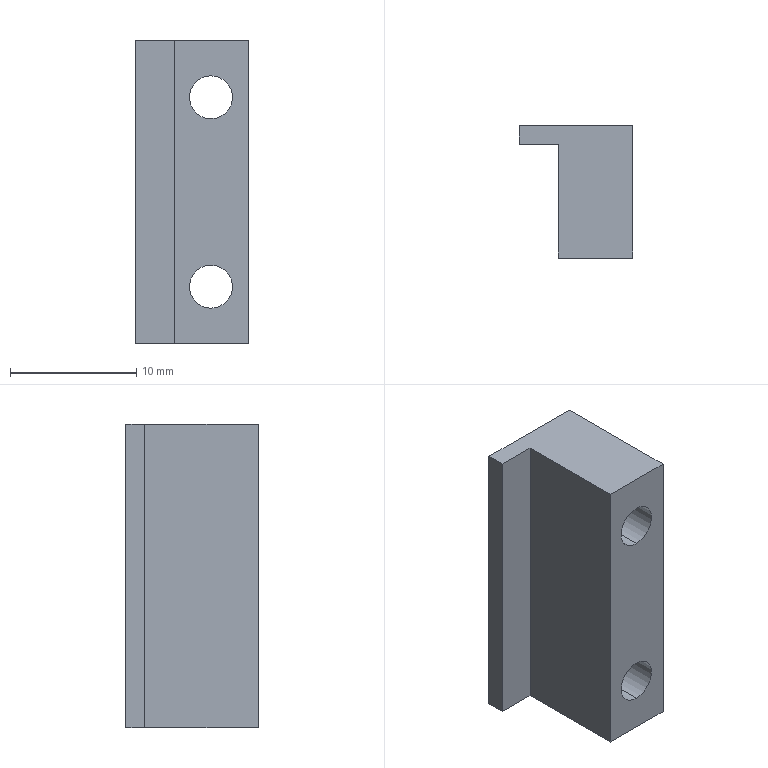Part | STEP file | PN_0016 | 1 solid | 12 faces | box 9 x 10.5 x 24 mm | volume 1408 mm3 | plane 8 | cylinder 4 | commonest cylinder face diameters 3.4 x4
STEP:
#1=CARTESIAN_POINT('',(0.,0.,0.));
#2=DIRECTION('',(0.,0.,1.));
#3=DIRECTION('',(1.,0.,0.));
#4=AXIS2_PLACEMENT_3D('',#1,#2,#3);
#5=CARTESIAN_POINT('',(1.5,0.,-5.8));
#6=VERTEX_POINT('',#5);
#7=CARTESIAN_POINT('',(1.5,10.5,-5.8));
#8=VERTEX_POINT('',#7);
#9=CARTESIAN_POINT('',(1.5,10.5,-5.8));
#10=DIRECTION('',(0.,1.,0.));
#11=VECTOR('',#10,1.);
#12=LINE('',#9,#11);
#13=CARTESIAN_POINT('',(1.5,10.5,-7.5));
#14=DIRECTION('',(0.,1.,0.));
#15=DIRECTION('',(0.,0.,1.));
#16=AXIS2_PLACEMENT_3D('',#13,#14,#15);
#17=CYLINDRICAL_SURFACE('',#16,1.7);
#18=CARTESIAN_POINT('',(6.283,0.));
#19=DIRECTION('',(0.,1.));
#20=VECTOR('',#19,1.);
#21=LINE('',#18,#20);
#22=(GEOMETRIC_REPRESENTATION_CONTEXT(2)PARAMETRIC_REPRESENTATION_CONTEXT()REPRESENTATION_CONTEXT('',''));
#23=DEFINITIONAL_REPRESENTATION('',(#21),#22);
#24=PCURVE('',#17,#23);
#25=CARTESIAN_POINT('',(1.5,10.5,-7.5));
#26=DIRECTION('',(0.,1.,0.));
#27=DIRECTION('',(0.,0.,1.));
#28=AXIS2_PLACEMENT_3D('',#25,#26,#27);
#29=CYLINDRICAL_SURFACE('',#28,1.7);
#30=CARTESIAN_POINT('',(0.,0.));
#31=DIRECTION('',(0.,1.));
#32=VECTOR('',#31,1.);
#33=LINE('',#30,#32);
#34=(GEOMETRIC_REPRESENTATION_CONTEXT(2)PARAMETRIC_REPRESENTATION_CONTEXT()REPRESENTATION_CONTEXT('',''));
#35=DEFINITIONAL_REPRESENTATION('',(#33),#34);
#36=PCURVE('',#29,#35);
#37=SURFACE_CURVE('',#12,(#24,#36),.PCURVE_S1.);
#38=EDGE_CURVE('',#6,#8,#37,.T.);
#39=ORIENTED_EDGE('',*,*,#38,.T.);
#40=CARTESIAN_POINT('',(1.5,10.5,-9.2));
#41=VERTEX_POINT('',#40);
#42=CARTESIAN_POINT('',(1.5,10.5,-7.5));
#43=DIRECTION('',(0.,1.,0.));
#44=DIRECTION('',(0.,0.,1.));
#45=AXIS2_PLACEMENT_3D('',#42,#43,#44);
#46=CIRCLE('',#45,1.7);
#47=CARTESIAN_POINT('',(0.,0.));
#48=DIRECTION('',(1.,0.));
#49=VECTOR('',#48,1.);
#50=LINE('',#47,#49);
#51=(GEOMETRIC_REPRESENTATION_CONTEXT(2)PARAMETRIC_REPRESENTATION_CONTEXT()REPRESENTATION_CONTEXT('',''));
#52=DEFINITIONAL_REPRESENTATION('',(#50),#51);
#53=PCURVE('',#17,#52);
#54=CARTESIAN_POINT('',(0.,10.5,0.));
#55=DIRECTION('',(0.,1.,0.));
#56=DIRECTION('',(0.,0.,1.));
#57=AXIS2_PLACEMENT_3D('',#54,#55,#56);
#58=PLANE('',#57);
#59=CARTESIAN_POINT('',(-7.5,1.5));
#60=DIRECTION('',(1.,0.));
#61=AXIS2_PLACEMENT_2D('',#59,#60);
#62=CIRCLE('',#61,1.7);
#63=(GEOMETRIC_REPRESENTATION_CONTEXT(2)PARAMETRIC_REPRESENTATION_CONTEXT()REPRESENTATION_CONTEXT('',''));
#64=DEFINITIONAL_REPRESENTATION('',(#62),#63);
#65=PCURVE('',#58,#64);
#66=SURFACE_CURVE('',#46,(#53,#65),.PCURVE_S1.);
#67=EDGE_CURVE('',#41,#8,#66,.T.);
#68=ORIENTED_EDGE('',*,*,#67,.F.);
#69=CARTESIAN_POINT('',(1.5,0.,-9.2));
#70=VERTEX_POINT('',#69);
#71=CARTESIAN_POINT('',(1.5,10.5,-9.2));
#72=DIRECTION('',(0.,1.,0.));
#73=VECTOR('',#72,1.);
#74=LINE('',#71,#73);
#75=CARTESIAN_POINT('',(3.142,0.));
#76=DIRECTION('',(0.,1.));
#77=VECTOR('',#76,1.);
#78=LINE('',#75,#77);
#79=(GEOMETRIC_REPRESENTATION_CONTEXT(2)PARAMETRIC_REPRESENTATION_CONTEXT()REPRESENTATION_CONTEXT('',''));
#80=DEFINITIONAL_REPRESENTATION('',(#78),#79);
#81=PCURVE('',#17,#80);
#82=CARTESIAN_POINT('',(3.142,0.));
#83=DIRECTION('',(0.,1.));
#84=VECTOR('',#83,1.);
#85=LINE('',#82,#84);
#86=(GEOMETRIC_REPRESENTATION_CONTEXT(2)PARAMETRIC_REPRESENTATION_CONTEXT()REPRESENTATION_CONTEXT('',''));
#87=DEFINITIONAL_REPRESENTATION('',(#85),#86);
#88=PCURVE('',#29,#87);
#89=SURFACE_CURVE('',#74,(#81,#88),.PCURVE_S1.);
#90=EDGE_CURVE('',#70,#41,#89,.T.);
#91=ORIENTED_EDGE('',*,*,#90,.F.);
#92=CARTESIAN_POINT('',(1.5,0.,-7.5));
#93=DIRECTION('',(0.,1.,0.));
#94=DIRECTION('',(0.,0.,1.));
#95=AXIS2_PLACEMENT_3D('',#92,#93,#94);
#96=CIRCLE('',#95,1.7);
#97=CARTESIAN_POINT('',(0.,-10.5));
#98=DIRECTION('',(1.,0.));
#99=VECTOR('',#98,1.);
#100=LINE('',#97,#99);
#101=(GEOMETRIC_REPRESENTATION_CONTEXT(2)PARAMETRIC_REPRESENTATION_CONTEXT()REPRESENTATION_CONTEXT('',''));
#102=DEFINITIONAL_REPRESENTATION('',(#100),#101);
#103=PCURVE('',#17,#102);
#104=CARTESIAN_POINT('',(0.,0.,0.));
#105=DIRECTION('',(0.,1.,0.));
#106=DIRECTION('',(0.,0.,1.));
#107=AXIS2_PLACEMENT_3D('',#104,#105,#106);
#108=PLANE('',#107);
#109=CARTESIAN_POINT('',(-7.5,1.5));
#110=DIRECTION('',(1.,0.));
#111=AXIS2_PLACEMENT_2D('',#109,#110);
#112=CIRCLE('',#111,1.7);
#113=(GEOMETRIC_REPRESENTATION_CONTEXT(2)PARAMETRIC_REPRESENTATION_CONTEXT()REPRESENTATION_CONTEXT('',''));
#114=DEFINITIONAL_REPRESENTATION('',(#112),#113);
#115=PCURVE('',#108,#114);
#116=SURFACE_CURVE('',#96,(#103,#115),.PCURVE_S1.);
#117=EDGE_CURVE('',#70,#6,#116,.T.);
#118=ORIENTED_EDGE('',*,*,#117,.T.);
#119=EDGE_LOOP('',(#39,#68,#91,#118));
#120=FACE_BOUND('',#119,.F.);
#121=ADVANCED_FACE('',(#120),#17,.F.);
#122=CARTESIAN_POINT('',(1.5,0.,9.2));
#123=VERTEX_POINT('',#122);
#124=CARTESIAN_POINT('',(1.5,10.5,9.2));
#125=VERTEX_POINT('',#124);
#126=CARTESIAN_POINT('',(1.5,10.5,9.2));
#127=DIRECTION('',(0.,1.,0.));
#128=VECTOR('',#127,1.);
#129=LINE('',#126,#128);
#130=CARTESIAN_POINT('',(1.5,10.5,7.5));
#131=DIRECTION('',(0.,1.,0.));
#132=DIRECTION('',(0.,0.,1.));
#133=AXIS2_PLACEMENT_3D('',#130,#131,#132);
#134=CYLINDRICAL_SURFACE('',#133,1.7);
#135=CARTESIAN_POINT('',(6.283,0.));
#136=DIRECTION('',(0.,1.));
#137=VECTOR('',#136,1.);
#138=LINE('',#135,#137);
#139=(GEOMETRIC_REPRESENTATION_CONTEXT(2)PARAMETRIC_REPRESENTATION_CONTEXT()REPRESENTATION_CONTEXT('',''));
#140=DEFINITIONAL_REPRESENTATION('',(#138),#139);
#141=PCURVE('',#134,#140);
#142=CARTESIAN_POINT('',(1.5,10.5,7.5));
#143=DIRECTION('',(0.,1.,0.));
#144=DIRECTION('',(0.,0.,1.));
#145=AXIS2_PLACEMENT_3D('',#142,#143,#144);
#146=CYLINDRICAL_SURFACE('',#145,1.7);
#147=CARTESIAN_POINT('',(0.,0.));
#148=DIRECTION('',(0.,1.));
#149=VECTOR('',#148,1.);
#150=LINE('',#147,#149);
#151=(GEOMETRIC_REPRESENTATION_CONTEXT(2)PARAMETRIC_REPRESENTATION_CONTEXT()REPRESENTATION_CONTEXT('',''));
#152=DEFINITIONAL_REPRESENTATION('',(#150),#151);
#153=PCURVE('',#146,#152);
#154=SURFACE_CURVE('',#129,(#141,#153),.PCURVE_S1.);
#155=EDGE_CURVE('',#123,#125,#154,.T.);
#156=ORIENTED_EDGE('',*,*,#155,.T.);
#157=CARTESIAN_POINT('',(1.5,10.5,5.8));
#158=VERTEX_POINT('',#157);
#159=CARTESIAN_POINT('',(1.5,10.5,7.5));
#160=DIRECTION('',(0.,1.,0.));
#161=DIRECTION('',(0.,0.,1.));
#162=AXIS2_PLACEMENT_3D('',#159,#160,#161);
#163=CIRCLE('',#162,1.7);
#164=CARTESIAN_POINT('',(0.,0.));
#165=DIRECTION('',(1.,0.));
#166=VECTOR('',#165,1.);
#167=LINE('',#164,#166);
#168=(GEOMETRIC_REPRESENTATION_CONTEXT(2)PARAMETRIC_REPRESENTATION_CONTEXT()REPRESENTATION_CONTEXT('',''));
#169=DEFINITIONAL_REPRESENTATION('',(#167),#168);
#170=PCURVE('',#134,#169);
#171=CARTESIAN_POINT('',(7.5,1.5));
#172=DIRECTION('',(1.,0.));
#173=AXIS2_PLACEMENT_2D('',#171,#172);
#174=CIRCLE('',#173,1.7);
#175=(GEOMETRIC_REPRESENTATION_CONTEXT(2)PARAMETRIC_REPRESENTATION_CONTEXT()REPRESENTATION_CONTEXT('',''));
#176=DEFINITIONAL_REPRESENTATION('',(#174),#175);
#177=PCURVE('',#58,#176);
#178=SURFACE_CURVE('',#163,(#170,#177),.PCURVE_S1.);
#179=EDGE_CURVE('',#158,#125,#178,.T.);
#180=ORIENTED_EDGE('',*,*,#179,.F.);
#181=CARTESIAN_POINT('',(1.5,0.,5.8));
#182=VERTEX_POINT('',#181);
#183=CARTESIAN_POINT('',(1.5,10.5,5.8));
#184=DIRECTION('',(0.,1.,0.));
#185=VECTOR('',#184,1.);
#186=LINE('',#183,#185);
#187=CARTESIAN_POINT('',(3.142,0.));
#188=DIRECTION('',(0.,1.));
#189=VECTOR('',#188,1.);
#190=LINE('',#187,#189);
#191=(GEOMETRIC_REPRESENTATION_CONTEXT(2)PARAMETRIC_REPRESENTATION_CONTEXT()REPRESENTATION_CONTEXT('',''));
#192=DEFINITIONAL_REPRESENTATION('',(#190),#191);
#193=PCURVE('',#134,#192);
#194=CARTESIAN_POINT('',(3.142,0.));
#195=DIRECTION('',(0.,1.));
#196=VECTOR('',#195,1.);
#197=LINE('',#194,#196);
#198=(GEOMETRIC_REPRESENTATION_CONTEXT(2)PARAMETRIC_REPRESENTATION_CONTEXT()REPRESENTATION_CONTEXT('',''));
#199=DEFINITIONAL_REPRESENTATION('',(#197),#198);
#200=PCURVE('',#146,#199);
#201=SURFACE_CURVE('',#186,(#193,#200),.PCURVE_S1.);
#202=EDGE_CURVE('',#182,#158,#201,.T.);
#203=ORIENTED_EDGE('',*,*,#202,.F.);
#204=CARTESIAN_POINT('',(1.5,0.,7.5));
#205=DIRECTION('',(0.,1.,0.));
#206=DIRECTION('',(0.,0.,1.));
#207=AXIS2_PLACEMENT_3D('',#204,#205,#206);
#208=CIRCLE('',#207,1.7);
#209=CARTESIAN_POINT('',(0.,-10.5));
#210=DIRECTION('',(1.,0.));
#211=VECTOR('',#210,1.);
#212=LINE('',#209,#211);
#213=(GEOMETRIC_REPRESENTATION_CONTEXT(2)PARAMETRIC_REPRESENTATION_CONTEXT()REPRESENTATION_CONTEXT('',''));
#214=DEFINITIONAL_REPRESENTATION('',(#212),#213);
#215=PCURVE('',#134,#214);
#216=CARTESIAN_POINT('',(7.5,1.5));
#217=DIRECTION('',(1.,0.));
#218=AXIS2_PLACEMENT_2D('',#216,#217);
#219=CIRCLE('',#218,1.7);
#220=(GEOMETRIC_REPRESENTATION_CONTEXT(2)PARAMETRIC_REPRESENTATION_CONTEXT()REPRESENTATION_CONTEXT('',''));
#221=DEFINITIONAL_REPRESENTATION('',(#219),#220);
#222=PCURVE('',#108,#221);
#223=SURFACE_CURVE('',#208,(#215,#222),.PCURVE_S1.);
#224=EDGE_CURVE('',#182,#123,#223,.T.);
#225=ORIENTED_EDGE('',*,*,#224,.T.);
#226=EDGE_LOOP('',(#156,#180,#203,#225));
#227=FACE_BOUND('',#226,.F.);
#228=ADVANCED_FACE('',(#227),#134,.F.);
#229=CARTESIAN_POINT('',(4.5,0.,12.));
#230=VERTEX_POINT('',#229);
#231=CARTESIAN_POINT('',(4.5,0.,-12.));
#232=VERTEX_POINT('',#231);
#233=CARTESIAN_POINT('',(4.5,0.,-12.));
#234=DIRECTION('',(0.,0.,-1.));
#235=VECTOR('',#234,1.);
#236=LINE('',#233,#235);
#237=CARTESIAN_POINT('',(4.5,10.5,-12.));
#238=DIRECTION('',(-1.,0.,0.));
#239=DIRECTION('',(0.,0.,1.));
#240=AXIS2_PLACEMENT_3D('',#237,#238,#239);
#241=PLANE('',#240);
#242=CARTESIAN_POINT('',(0.,-10.5));
#243=DIRECTION('',(-1.,0.));
#244=VECTOR('',#243,1.);
#245=LINE('',#242,#244);
#246=(GEOMETRIC_REPRESENTATION_CONTEXT(2)PARAMETRIC_REPRESENTATION_CONTEXT()REPRESENTATION_CONTEXT('',''));
#247=DEFINITIONAL_REPRESENTATION('',(#245),#246);
#248=PCURVE('',#241,#247);
#249=CARTESIAN_POINT('',(-12.,4.5));
#250=DIRECTION('',(-1.,0.));
#251=VECTOR('',#250,1.);
#252=LINE('',#249,#251);
#253=(GEOMETRIC_REPRESENTATION_CONTEXT(2)PARAMETRIC_REPRESENTATION_CONTEXT()REPRESENTATION_CONTEXT('',''));
#254=DEFINITIONAL_REPRESENTATION('',(#252),#253);
#255=PCURVE('',#108,#254);
#256=SURFACE_CURVE('',#236,(#248,#255),.PCURVE_S1.);
#257=EDGE_CURVE('',#230,#232,#256,.T.);
#258=ORIENTED_EDGE('',*,*,#257,.T.);
#259=CARTESIAN_POINT('',(4.5,10.5,-12.));
#260=VERTEX_POINT('',#259);
#261=CARTESIAN_POINT('',(4.5,10.5,-12.));
#262=DIRECTION('',(0.,-1.,0.));
#263=VECTOR('',#262,1.);
#264=LINE('',#261,#263);
#265=CARTESIAN_POINT('',(0.,0.));
#266=DIRECTION('',(0.,-1.));
#267=VECTOR('',#266,1.);
#268=LINE('',#265,#267);
#269=(GEOMETRIC_REPRESENTATION_CONTEXT(2)PARAMETRIC_REPRESENTATION_CONTEXT()REPRESENTATION_CONTEXT('',''));
#270=DEFINITIONAL_REPRESENTATION('',(#268),#269);
#271=PCURVE('',#241,#270);
#272=CARTESIAN_POINT('',(-4.5,10.5,-12.));
#273=DIRECTION('',(0.,0.,1.));
#274=DIRECTION('',(1.,0.,0.));
#275=AXIS2_PLACEMENT_3D('',#272,#273,#274);
#276=PLANE('',#275);
#277=CARTESIAN_POINT('',(9.,0.));
#278=DIRECTION('',(0.,-1.));
#279=VECTOR('',#278,1.);
#280=LINE('',#277,#279);
#281=(GEOMETRIC_REPRESENTATION_CONTEXT(2)PARAMETRIC_REPRESENTATION_CONTEXT()REPRESENTATION_CONTEXT('',''));
#282=DEFINITIONAL_REPRESENTATION('',(#280),#281);
#283=PCURVE('',#276,#282);
#284=SURFACE_CURVE('',#264,(#271,#283),.PCURVE_S1.);
#285=EDGE_CURVE('',#260,#232,#284,.T.);
#286=ORIENTED_EDGE('',*,*,#285,.F.);
#287=CARTESIAN_POINT('',(4.5,10.5,12.));
#288=VERTEX_POINT('',#287);
#289=CARTESIAN_POINT('',(4.5,10.5,-12.));
#290=DIRECTION('',(0.,0.,-1.));
#291=VECTOR('',#290,1.);
#292=LINE('',#289,#291);
#293=CARTESIAN_POINT('',(0.,0.));
#294=DIRECTION('',(-1.,0.));
#295=VECTOR('',#294,1.);
#296=LINE('',#293,#295);
#297=(GEOMETRIC_REPRESENTATION_CONTEXT(2)PARAMETRIC_REPRESENTATION_CONTEXT()REPRESENTATION_CONTEXT('',''));
#298=DEFINITIONAL_REPRESENTATION('',(#296),#297);
#299=PCURVE('',#241,#298);
#300=CARTESIAN_POINT('',(-12.,4.5));
#301=DIRECTION('',(-1.,0.));
#302=VECTOR('',#301,1.);
#303=LINE('',#300,#302);
#304=(GEOMETRIC_REPRESENTATION_CONTEXT(2)PARAMETRIC_REPRESENTATION_CONTEXT()REPRESENTATION_CONTEXT('',''));
#305=DEFINITIONAL_REPRESENTATION('',(#303),#304);
#306=PCURVE('',#58,#305);
#307=SURFACE_CURVE('',#292,(#299,#306),.PCURVE_S1.);
#308=EDGE_CURVE('',#288,#260,#307,.T.);
#309=ORIENTED_EDGE('',*,*,#308,.F.);
#310=CARTESIAN_POINT('',(4.5,10.5,12.));
#311=DIRECTION('',(0.,-1.,0.));
#312=VECTOR('',#311,1.);
#313=LINE('',#310,#312);
#314=CARTESIAN_POINT('',(24.,0.));
#315=DIRECTION('',(0.,-1.));
#316=VECTOR('',#315,1.);
#317=LINE('',#314,#316);
#318=(GEOMETRIC_REPRESENTATION_CONTEXT(2)PARAMETRIC_REPRESENTATION_CONTEXT()REPRESENTATION_CONTEXT('',''));
#319=DEFINITIONAL_REPRESENTATION('',(#317),#318);
#320=PCURVE('',#241,#319);
#321=CARTESIAN_POINT('',(-4.5,10.5,12.));
#322=DIRECTION('',(0.,0.,-1.));
#323=DIRECTION('',(-1.,0.,0.));
#324=AXIS2_PLACEMENT_3D('',#321,#322,#323);
#325=PLANE('',#324);
#326=CARTESIAN_POINT('',(-9.,0.));
#327=DIRECTION('',(0.,-1.));
#328=VECTOR('',#327,1.);
#329=LINE('',#326,#328);
#330=(GEOMETRIC_REPRESENTATION_CONTEXT(2)PARAMETRIC_REPRESENTATION_CONTEXT()REPRESENTATION_CONTEXT('',''));
#331=DEFINITIONAL_REPRESENTATION('',(#329),#330);
#332=PCURVE('',#325,#331);
#333=SURFACE_CURVE('',#313,(#320,#332),.PCURVE_S1.);
#334=EDGE_CURVE('',#288,#230,#333,.T.);
#335=ORIENTED_EDGE('',*,*,#334,.T.);
#336=EDGE_LOOP('',(#258,#286,#309,#335));
#337=FACE_BOUND('',#336,.T.);
#338=ADVANCED_FACE('',(#337),#241,.F.);
#339=CARTESIAN_POINT('',(-1.4,0.,-12.));
#340=VERTEX_POINT('',#339);
#341=CARTESIAN_POINT('',(-1.4,9.,-12.));
#342=VERTEX_POINT('',#341);
#343=CARTESIAN_POINT('',(-1.4,0.,-12.));
#344=DIRECTION('',(0.,1.,0.));
#345=VECTOR('',#344,1.);
#346=LINE('',#343,#345);
#347=CARTESIAN_POINT('',(3.1,-10.5));
#348=DIRECTION('',(0.,1.));
#349=VECTOR('',#348,1.);
#350=LINE('',#347,#349);
#351=(GEOMETRIC_REPRESENTATION_CONTEXT(2)PARAMETRIC_REPRESENTATION_CONTEXT()REPRESENTATION_CONTEXT('',''));
#352=DEFINITIONAL_REPRESENTATION('',(#350),#351);
#353=PCURVE('',#276,#352);
#354=CARTESIAN_POINT('',(-1.4,0.,-12.));
#355=DIRECTION('',(1.,0.,0.));
#356=DIRECTION('',(0.,0.,-1.));
#357=AXIS2_PLACEMENT_3D('',#354,#355,#356);
#358=PLANE('',#357);
#359=CARTESIAN_POINT('',(0.,0.));
#360=DIRECTION('',(0.,1.));
#361=VECTOR('',#360,1.);
#362=LINE('',#359,#361);
#363=(GEOMETRIC_REPRESENTATION_CONTEXT(2)PARAMETRIC_REPRESENTATION_CONTEXT()REPRESENTATION_CONTEXT('',''));
#364=DEFINITIONAL_REPRESENTATION('',(#362),#363);
#365=PCURVE('',#358,#364);
#366=SURFACE_CURVE('',#346,(#353,#365),.PCURVE_S1.);
#367=EDGE_CURVE('',#340,#342,#366,.T.);
#368=ORIENTED_EDGE('',*,*,#367,.T.);
#369=CARTESIAN_POINT('',(-4.5,9.,-12.));
#370=VERTEX_POINT('',#369);
#371=CARTESIAN_POINT('',(-4.5,9.,-12.));
#372=DIRECTION('',(-1.,0.,0.));
#373=VECTOR('',#372,1.);
#374=LINE('',#371,#373);
#375=CARTESIAN_POINT('',(0.,-1.5));
#376=DIRECTION('',(-1.,0.));
#377=VECTOR('',#376,1.);
#378=LINE('',#375,#377);
#379=(GEOMETRIC_REPRESENTATION_CONTEXT(2)PARAMETRIC_REPRESENTATION_CONTEXT()REPRESENTATION_CONTEXT('',''));
#380=DEFINITIONAL_REPRESENTATION('',(#378),#379);
#381=PCURVE('',#276,#380);
#382=CARTESIAN_POINT('',(-4.5,9.,-12.));
#383=DIRECTION('',(0.,1.,0.));
#384=DIRECTION('',(0.,0.,1.));
#385=AXIS2_PLACEMENT_3D('',#382,#383,#384);
#386=PLANE('',#385);
#387=CARTESIAN_POINT('',(0.,0.));
#388=DIRECTION('',(0.,-1.));
#389=VECTOR('',#388,1.);
#390=LINE('',#387,#389);
#391=(GEOMETRIC_REPRESENTATION_CONTEXT(2)PARAMETRIC_REPRESENTATION_CONTEXT()REPRESENTATION_CONTEXT('',''));
#392=DEFINITIONAL_REPRESENTATION('',(#390),#391);
#393=PCURVE('',#386,#392);
#394=SURFACE_CURVE('',#374,(#381,#393),.PCURVE_S1.);
#395=EDGE_CURVE('',#342,#370,#394,.T.);
#396=ORIENTED_EDGE('',*,*,#395,.T.);
#397=CARTESIAN_POINT('',(-4.5,10.5,-12.));
#398=VERTEX_POINT('',#397);
#399=CARTESIAN_POINT('',(-4.5,10.5,-12.));
#400=DIRECTION('',(0.,-1.,0.));
#401=VECTOR('',#400,1.);
#402=LINE('',#399,#401);
#403=CARTESIAN_POINT('',(0.,0.));
#404=DIRECTION('',(0.,-1.));
#405=VECTOR('',#404,1.);
#406=LINE('',#403,#405);
#407=(GEOMETRIC_REPRESENTATION_CONTEXT(2)PARAMETRIC_REPRESENTATION_CONTEXT()REPRESENTATION_CONTEXT('',''));
#408=DEFINITIONAL_REPRESENTATION('',(#406),#407);
#409=PCURVE('',#276,#408);
#410=CARTESIAN_POINT('',(-4.5,10.5,-12.));
#411=DIRECTION('',(1.,0.,0.));
#412=DIRECTION('',(0.,0.,-1.));
#413=AXIS2_PLACEMENT_3D('',#410,#411,#412);
#414=PLANE('',#413);
#415=CARTESIAN_POINT('',(0.,0.));
#416=DIRECTION('',(0.,-1.));
#417=VECTOR('',#416,1.);
#418=LINE('',#415,#417);
#419=(GEOMETRIC_REPRESENTATION_CONTEXT(2)PARAMETRIC_REPRESENTATION_CONTEXT()REPRESENTATION_CONTEXT('',''));
#420=DEFINITIONAL_REPRESENTATION('',(#418),#419);
#421=PCURVE('',#414,#420);
#422=SURFACE_CURVE('',#402,(#409,#421),.PCURVE_S1.);
#423=EDGE_CURVE('',#398,#370,#422,.T.);
#424=ORIENTED_EDGE('',*,*,#423,.F.);
#425=CARTESIAN_POINT('',(-4.5,10.5,-12.));
#426=DIRECTION('',(-1.,0.,0.));
#427=VECTOR('',#426,1.);
#428=LINE('',#425,#427);
#429=CARTESIAN_POINT('',(0.,0.));
#430=DIRECTION('',(-1.,0.));
#431=VECTOR('',#430,1.);
#432=LINE('',#429,#431);
#433=(GEOMETRIC_REPRESENTATION_CONTEXT(2)PARAMETRIC_REPRESENTATION_CONTEXT()REPRESENTATION_CONTEXT('',''));
#434=DEFINITIONAL_REPRESENTATION('',(#432),#433);
#435=PCURVE('',#276,#434);
#436=CARTESIAN_POINT('',(-12.,-4.5));
#437=DIRECTION('',(0.,-1.));
#438=VECTOR('',#437,1.);
#439=LINE('',#436,#438);
#440=(GEOMETRIC_REPRESENTATION_CONTEXT(2)PARAMETRIC_REPRESENTATION_CONTEXT()REPRESENTATION_CONTEXT('',''));
#441=DEFINITIONAL_REPRESENTATION('',(#439),#440);
#442=PCURVE('',#58,#441);
#443=SURFACE_CURVE('',#428,(#435,#442),.PCURVE_S1.);
#444=EDGE_CURVE('',#260,#398,#443,.T.);
#445=ORIENTED_EDGE('',*,*,#444,.F.);
#446=ORIENTED_EDGE('',*,*,#285,.T.);
#447=CARTESIAN_POINT('',(-4.5,0.,-12.));
#448=DIRECTION('',(-1.,0.,0.));
#449=VECTOR('',#448,1.);
#450=LINE('',#447,#449);
#451=CARTESIAN_POINT('',(0.,-10.5));
#452=DIRECTION('',(-1.,0.));
#453=VECTOR('',#452,1.);
#454=LINE('',#451,#453);
#455=(GEOMETRIC_REPRESENTATION_CONTEXT(2)PARAMETRIC_REPRESENTATION_CONTEXT()REPRESENTATION_CONTEXT('',''));
#456=DEFINITIONAL_REPRESENTATION('',(#454),#455);
#457=PCURVE('',#276,#456);
#458=CARTESIAN_POINT('',(-12.,-4.5));
#459=DIRECTION('',(0.,-1.));
#460=VECTOR('',#459,1.);
#461=LINE('',#458,#460);
#462=(GEOMETRIC_REPRESENTATION_CONTEXT(2)PARAMETRIC_REPRESENTATION_CONTEXT()REPRESENTATION_CONTEXT('',''));
#463=DEFINITIONAL_REPRESENTATION('',(#461),#462);
#464=PCURVE('',#108,#463);
#465=SURFACE_CURVE('',#450,(#457,#464),.PCURVE_S1.);
#466=EDGE_CURVE('',#232,#340,#465,.T.);
#467=ORIENTED_EDGE('',*,*,#466,.T.);
#468=EDGE_LOOP('',(#368,#396,#424,#445,#446,#467));
#469=FACE_BOUND('',#468,.T.);
#470=ADVANCED_FACE('',(#469),#276,.F.);
#471=ORIENTED_EDGE('',*,*,#423,.T.);
#472=CARTESIAN_POINT('',(-4.5,9.,12.));
#473=VERTEX_POINT('',#472);
#474=CARTESIAN_POINT('',(-4.5,9.,-12.));
#475=DIRECTION('',(0.,0.,1.));
#476=VECTOR('',#475,1.);
#477=LINE('',#474,#476);
#478=CARTESIAN_POINT('',(0.,-1.5));
#479=DIRECTION('',(-1.,0.));
#480=VECTOR('',#479,1.);
#481=LINE('',#478,#480);
#482=(GEOMETRIC_REPRESENTATION_CONTEXT(2)PARAMETRIC_REPRESENTATION_CONTEXT()REPRESENTATION_CONTEXT('',''));
#483=DEFINITIONAL_REPRESENTATION('',(#481),#482);
#484=PCURVE('',#414,#483);
#485=CARTESIAN_POINT('',(0.,0.));
#486=DIRECTION('',(1.,0.));
#487=VECTOR('',#486,1.);
#488=LINE('',#485,#487);
#489=(GEOMETRIC_REPRESENTATION_CONTEXT(2)PARAMETRIC_REPRESENTATION_CONTEXT()REPRESENTATION_CONTEXT('',''));
#490=DEFINITIONAL_REPRESENTATION('',(#488),#489);
#491=PCURVE('',#386,#490);
#492=SURFACE_CURVE('',#477,(#484,#491),.PCURVE_S1.);
#493=EDGE_CURVE('',#370,#473,#492,.T.);
#494=ORIENTED_EDGE('',*,*,#493,.T.);
#495=CARTESIAN_POINT('',(-4.5,10.5,12.));
#496=VERTEX_POINT('',#495);
#497=CARTESIAN_POINT('',(-4.5,10.5,12.));
#498=DIRECTION('',(0.,-1.,0.));
#499=VECTOR('',#498,1.);
#500=LINE('',#497,#499);
#501=CARTESIAN_POINT('',(-24.,0.));
#502=DIRECTION('',(0.,-1.));
#503=VECTOR('',#502,1.);
#504=LINE('',#501,#503);
#505=(GEOMETRIC_REPRESENTATION_CONTEXT(2)PARAMETRIC_REPRESENTATION_CONTEXT()REPRESENTATION_CONTEXT('',''));
#506=DEFINITIONAL_REPRESENTATION('',(#504),#505);
#507=PCURVE('',#414,#506);
#508=CARTESIAN_POINT('',(0.,0.));
#509=DIRECTION('',(0.,-1.));
#510=VECTOR('',#509,1.);
#511=LINE('',#508,#510);
#512=(GEOMETRIC_REPRESENTATION_CONTEXT(2)PARAMETRIC_REPRESENTATION_CONTEXT()REPRESENTATION_CONTEXT('',''));
#513=DEFINITIONAL_REPRESENTATION('',(#511),#512);
#514=PCURVE('',#325,#513);
#515=SURFACE_CURVE('',#500,(#507,#514),.PCURVE_S1.);
#516=EDGE_CURVE('',#496,#473,#515,.T.);
#517=ORIENTED_EDGE('',*,*,#516,.F.);
#518=CARTESIAN_POINT('',(-4.5,10.5,-12.));
#519=DIRECTION('',(0.,0.,1.));
#520=VECTOR('',#519,1.);
#521=LINE('',#518,#520);
#522=CARTESIAN_POINT('',(0.,0.));
#523=DIRECTION('',(-1.,0.));
#524=VECTOR('',#523,1.);
#525=LINE('',#522,#524);
#526=(GEOMETRIC_REPRESENTATION_CONTEXT(2)PARAMETRIC_REPRESENTATION_CONTEXT()REPRESENTATION_CONTEXT('',''));
#527=DEFINITIONAL_REPRESENTATION('',(#525),#526);
#528=PCURVE('',#414,#527);
#529=CARTESIAN_POINT('',(-12.,-4.5));
#530=DIRECTION('',(1.,0.));
#531=VECTOR('',#530,1.);
#532=LINE('',#529,#531);
#533=(GEOMETRIC_REPRESENTATION_CONTEXT(2)PARAMETRIC_REPRESENTATION_CONTEXT()REPRESENTATION_CONTEXT('',''));
#534=DEFINITIONAL_REPRESENTATION('',(#532),#533);
#535=PCURVE('',#58,#534);
#536=SURFACE_CURVE('',#521,(#528,#535),.PCURVE_S1.);
#537=EDGE_CURVE('',#398,#496,#536,.T.);
#538=ORIENTED_EDGE('',*,*,#537,.F.);
#539=EDGE_LOOP('',(#471,#494,#517,#538));
#540=FACE_BOUND('',#539,.T.);
#541=ADVANCED_FACE('',(#540),#414,.F.);
#542=ORIENTED_EDGE('',*,*,#516,.T.);
#543=CARTESIAN_POINT('',(-1.4,9.,12.));
#544=VERTEX_POINT('',#543);
#545=CARTESIAN_POINT('',(-4.5,9.,12.));
#546=DIRECTION('',(-1.,0.,0.));
#547=VECTOR('',#546,1.);
#548=LINE('',#545,#547);
#549=CARTESIAN_POINT('',(0.,-1.5));
#550=DIRECTION('',(1.,0.));
#551=VECTOR('',#550,1.);
#552=LINE('',#549,#551);
#553=(GEOMETRIC_REPRESENTATION_CONTEXT(2)PARAMETRIC_REPRESENTATION_CONTEXT()REPRESENTATION_CONTEXT('',''));
#554=DEFINITIONAL_REPRESENTATION('',(#552),#553);
#555=PCURVE('',#325,#554);
#556=CARTESIAN_POINT('',(24.,0.));
#557=DIRECTION('',(0.,-1.));
#558=VECTOR('',#557,1.);
#559=LINE('',#556,#558);
#560=(GEOMETRIC_REPRESENTATION_CONTEXT(2)PARAMETRIC_REPRESENTATION_CONTEXT()REPRESENTATION_CONTEXT('',''));
#561=DEFINITIONAL_REPRESENTATION('',(#559),#560);
#562=PCURVE('',#386,#561);
#563=SURFACE_CURVE('',#548,(#555,#562),.PCURVE_S1.);
#564=EDGE_CURVE('',#544,#473,#563,.T.);
#565=ORIENTED_EDGE('',*,*,#564,.F.);
#566=CARTESIAN_POINT('',(-1.4,0.,12.));
#567=VERTEX_POINT('',#566);
#568=CARTESIAN_POINT('',(-1.4,0.,12.));
#569=DIRECTION('',(0.,1.,0.));
#570=VECTOR('',#569,1.);
#571=LINE('',#568,#570);
#572=CARTESIAN_POINT('',(-3.1,-10.5));
#573=DIRECTION('',(0.,1.));
#574=VECTOR('',#573,1.);
#575=LINE('',#572,#574);
#576=(GEOMETRIC_REPRESENTATION_CONTEXT(2)PARAMETRIC_REPRESENTATION_CONTEXT()REPRESENTATION_CONTEXT('',''));
#577=DEFINITIONAL_REPRESENTATION('',(#575),#576);
#578=PCURVE('',#325,#577);
#579=CARTESIAN_POINT('',(-24.,0.));
#580=DIRECTION('',(0.,1.));
#581=VECTOR('',#580,1.);
#582=LINE('',#579,#581);
#583=(GEOMETRIC_REPRESENTATION_CONTEXT(2)PARAMETRIC_REPRESENTATION_CONTEXT()REPRESENTATION_CONTEXT('',''));
#584=DEFINITIONAL_REPRESENTATION('',(#582),#583);
#585=PCURVE('',#358,#584);
#586=SURFACE_CURVE('',#571,(#578,#585),.PCURVE_S1.);
#587=EDGE_CURVE('',#567,#544,#586,.T.);
#588=ORIENTED_EDGE('',*,*,#587,.F.);
#589=CARTESIAN_POINT('',(-4.5,0.,12.));
#590=DIRECTION('',(1.,0.,0.));
#591=VECTOR('',#590,1.);
#592=LINE('',#589,#591);
#593=CARTESIAN_POINT('',(0.,-10.5));
#594=DIRECTION('',(-1.,0.));
#595=VECTOR('',#594,1.);
#596=LINE('',#593,#595);
#597=(GEOMETRIC_REPRESENTATION_CONTEXT(2)PARAMETRIC_REPRESENTATION_CONTEXT()REPRESENTATION_CONTEXT('',''));
#598=DEFINITIONAL_REPRESENTATION('',(#596),#597);
#599=PCURVE('',#325,#598);
#600=CARTESIAN_POINT('',(12.,-4.5));
#601=DIRECTION('',(0.,1.));
#602=VECTOR('',#601,1.);
#603=LINE('',#600,#602);
#604=(GEOMETRIC_REPRESENTATION_CONTEXT(2)PARAMETRIC_REPRESENTATION_CONTEXT()REPRESENTATION_CONTEXT('',''));
#605=DEFINITIONAL_REPRESENTATION('',(#603),#604);
#606=PCURVE('',#108,#605);
#607=SURFACE_CURVE('',#592,(#599,#606),.PCURVE_S1.);
#608=EDGE_CURVE('',#567,#230,#607,.T.);
#609=ORIENTED_EDGE('',*,*,#608,.T.);
#610=ORIENTED_EDGE('',*,*,#334,.F.);
#611=CARTESIAN_POINT('',(-4.5,10.5,12.));
#612=DIRECTION('',(1.,0.,0.));
#613=VECTOR('',#612,1.);
#614=LINE('',#611,#613);
#615=CARTESIAN_POINT('',(0.,0.));
#616=DIRECTION('',(-1.,0.));
#617=VECTOR('',#616,1.);
#618=LINE('',#615,#617);
#619=(GEOMETRIC_REPRESENTATION_CONTEXT(2)PARAMETRIC_REPRESENTATION_CONTEXT()REPRESENTATION_CONTEXT('',''));
#620=DEFINITIONAL_REPRESENTATION('',(#618),#619);
#621=PCURVE('',#325,#620);
#622=CARTESIAN_POINT('',(12.,-4.5));
#623=DIRECTION('',(0.,1.));
#624=VECTOR('',#623,1.);
#625=LINE('',#622,#624);
#626=(GEOMETRIC_REPRESENTATION_CONTEXT(2)PARAMETRIC_REPRESENTATION_CONTEXT()REPRESENTATION_CONTEXT('',''));
#627=DEFINITIONAL_REPRESENTATION('',(#625),#626);
#628=PCURVE('',#58,#627);
#629=SURFACE_CURVE('',#614,(#621,#628),.PCURVE_S1.);
#630=EDGE_CURVE('',#496,#288,#629,.T.);
#631=ORIENTED_EDGE('',*,*,#630,.F.);
#632=EDGE_LOOP('',(#542,#565,#588,#609,#610,#631));
#633=FACE_BOUND('',#632,.T.);
#634=ADVANCED_FACE('',(#633),#325,.F.);
#635=CARTESIAN_POINT('',(1.5,10.5,-7.5));
#636=DIRECTION('',(0.,1.,0.));
#637=DIRECTION('',(0.,0.,1.));
#638=AXIS2_PLACEMENT_3D('',#635,#636,#637);
#639=CIRCLE('',#638,1.7);
#640=CARTESIAN_POINT('',(-7.5,1.5));
#641=DIRECTION('',(1.,0.));
#642=AXIS2_PLACEMENT_2D('',#640,#641);
#643=CIRCLE('',#642,1.7);
#644=(GEOMETRIC_REPRESENTATION_CONTEXT(2)PARAMETRIC_REPRESENTATION_CONTEXT()REPRESENTATION_CONTEXT('',''));
#645=DEFINITIONAL_REPRESENTATION('',(#643),#644);
#646=PCURVE('',#58,#645);
#647=CARTESIAN_POINT('',(0.,0.));
#648=DIRECTION('',(1.,0.));
#649=VECTOR('',#648,1.);
#650=LINE('',#647,#649);
#651=(GEOMETRIC_REPRESENTATION_CONTEXT(2)PARAMETRIC_REPRESENTATION_CONTEXT()REPRESENTATION_CONTEXT('',''));
#652=DEFINITIONAL_REPRESENTATION('',(#650),#651);
#653=PCURVE('',#29,#652);
#654=SURFACE_CURVE('',#639,(#646,#653),.PCURVE_S1.);
#655=EDGE_CURVE('',#8,#41,#654,.T.);
#656=ORIENTED_EDGE('',*,*,#655,.F.);
#657=ORIENTED_EDGE('',*,*,#67,.F.);
#658=EDGE_LOOP('',(#656,#657));
#659=FACE_BOUND('',#658,.T.);
#660=CARTESIAN_POINT('',(1.5,10.5,7.5));
#661=DIRECTION('',(0.,1.,0.));
#662=DIRECTION('',(0.,0.,1.));
#663=AXIS2_PLACEMENT_3D('',#660,#661,#662);
#664=CIRCLE('',#663,1.7);
#665=CARTESIAN_POINT('',(7.5,1.5));
#666=DIRECTION('',(1.,0.));
#667=AXIS2_PLACEMENT_2D('',#665,#666);
#668=CIRCLE('',#667,1.7);
#669=(GEOMETRIC_REPRESENTATION_CONTEXT(2)PARAMETRIC_REPRESENTATION_CONTEXT()REPRESENTATION_CONTEXT('',''));
#670=DEFINITIONAL_REPRESENTATION('',(#668),#669);
#671=PCURVE('',#58,#670);
#672=CARTESIAN_POINT('',(0.,0.));
#673=DIRECTION('',(1.,0.));
#674=VECTOR('',#673,1.);
#675=LINE('',#672,#674);
#676=(GEOMETRIC_REPRESENTATION_CONTEXT(2)PARAMETRIC_REPRESENTATION_CONTEXT()REPRESENTATION_CONTEXT('',''));
#677=DEFINITIONAL_REPRESENTATION('',(#675),#676);
#678=PCURVE('',#146,#677);
#679=SURFACE_CURVE('',#664,(#671,#678),.PCURVE_S1.);
#680=EDGE_CURVE('',#125,#158,#679,.T.);
#681=ORIENTED_EDGE('',*,*,#680,.F.);
#682=ORIENTED_EDGE('',*,*,#179,.F.);
#683=EDGE_LOOP('',(#681,#682));
#684=FACE_BOUND('',#683,.T.);
#685=ORIENTED_EDGE('',*,*,#308,.T.);
#686=ORIENTED_EDGE('',*,*,#444,.T.);
#687=ORIENTED_EDGE('',*,*,#537,.T.);
#688=ORIENTED_EDGE('',*,*,#630,.T.);
#689=EDGE_LOOP('',(#685,#686,#687,#688));
#690=FACE_BOUND('',#689,.T.);
#691=ADVANCED_FACE('',(#659,#684,#690),#58,.T.);
#692=CARTESIAN_POINT('',(1.5,0.,-7.5));
#693=DIRECTION('',(0.,1.,0.));
#694=DIRECTION('',(0.,0.,1.));
#695=AXIS2_PLACEMENT_3D('',#692,#693,#694);
#696=CIRCLE('',#695,1.7);
#697=CARTESIAN_POINT('',(-7.5,1.5));
#698=DIRECTION('',(1.,0.));
#699=AXIS2_PLACEMENT_2D('',#697,#698);
#700=CIRCLE('',#699,1.7);
#701=(GEOMETRIC_REPRESENTATION_CONTEXT(2)PARAMETRIC_REPRESENTATION_CONTEXT()REPRESENTATION_CONTEXT('',''));
#702=DEFINITIONAL_REPRESENTATION('',(#700),#701);
#703=PCURVE('',#108,#702);
#704=CARTESIAN_POINT('',(0.,-10.5));
#705=DIRECTION('',(1.,0.));
#706=VECTOR('',#705,1.);
#707=LINE('',#704,#706);
#708=(GEOMETRIC_REPRESENTATION_CONTEXT(2)PARAMETRIC_REPRESENTATION_CONTEXT()REPRESENTATION_CONTEXT('',''));
#709=DEFINITIONAL_REPRESENTATION('',(#707),#708);
#710=PCURVE('',#29,#709);
#711=SURFACE_CURVE('',#696,(#703,#710),.PCURVE_S1.);
#712=EDGE_CURVE('',#6,#70,#711,.T.);
#713=ORIENTED_EDGE('',*,*,#712,.T.);
#714=ORIENTED_EDGE('',*,*,#117,.T.);
#715=EDGE_LOOP('',(#713,#714));
#716=FACE_BOUND('',#715,.T.);
#717=CARTESIAN_POINT('',(1.5,0.,7.5));
#718=DIRECTION('',(0.,1.,0.));
#719=DIRECTION('',(0.,0.,1.));
#720=AXIS2_PLACEMENT_3D('',#717,#718,#719);
#721=CIRCLE('',#720,1.7);
#722=CARTESIAN_POINT('',(7.5,1.5));
#723=DIRECTION('',(1.,0.));
#724=AXIS2_PLACEMENT_2D('',#722,#723);
#725=CIRCLE('',#724,1.7);
#726=(GEOMETRIC_REPRESENTATION_CONTEXT(2)PARAMETRIC_REPRESENTATION_CONTEXT()REPRESENTATION_CONTEXT('',''));
#727=DEFINITIONAL_REPRESENTATION('',(#725),#726);
#728=PCURVE('',#108,#727);
#729=CARTESIAN_POINT('',(0.,-10.5));
#730=DIRECTION('',(1.,0.));
#731=VECTOR('',#730,1.);
#732=LINE('',#729,#731);
#733=(GEOMETRIC_REPRESENTATION_CONTEXT(2)PARAMETRIC_REPRESENTATION_CONTEXT()REPRESENTATION_CONTEXT('',''));
#734=DEFINITIONAL_REPRESENTATION('',(#732),#733);
#735=PCURVE('',#146,#734);
#736=SURFACE_CURVE('',#721,(#728,#735),.PCURVE_S1.);
#737=EDGE_CURVE('',#123,#182,#736,.T.);
#738=ORIENTED_EDGE('',*,*,#737,.T.);
#739=ORIENTED_EDGE('',*,*,#224,.T.);
#740=EDGE_LOOP('',(#738,#739));
#741=FACE_BOUND('',#740,.T.);
#742=ORIENTED_EDGE('',*,*,#608,.F.);
#743=CARTESIAN_POINT('',(-1.4,0.,-12.));
#744=DIRECTION('',(0.,0.,1.));
#745=VECTOR('',#744,1.);
#746=LINE('',#743,#745);
#747=CARTESIAN_POINT('',(-12.,-1.4));
#748=DIRECTION('',(1.,0.));
#749=VECTOR('',#748,1.);
#750=LINE('',#747,#749);
#751=(GEOMETRIC_REPRESENTATION_CONTEXT(2)PARAMETRIC_REPRESENTATION_CONTEXT()REPRESENTATION_CONTEXT('',''));
#752=DEFINITIONAL_REPRESENTATION('',(#750),#751);
#753=PCURVE('',#108,#752);
#754=CARTESIAN_POINT('',(0.,0.));
#755=DIRECTION('',(-1.,0.));
#756=VECTOR('',#755,1.);
#757=LINE('',#754,#756);
#758=(GEOMETRIC_REPRESENTATION_CONTEXT(2)PARAMETRIC_REPRESENTATION_CONTEXT()REPRESENTATION_CONTEXT('',''));
#759=DEFINITIONAL_REPRESENTATION('',(#757),#758);
#760=PCURVE('',#358,#759);
#761=SURFACE_CURVE('',#746,(#753,#760),.PCURVE_S1.);
#762=EDGE_CURVE('',#340,#567,#761,.T.);
#763=ORIENTED_EDGE('',*,*,#762,.F.);
#764=ORIENTED_EDGE('',*,*,#466,.F.);
#765=ORIENTED_EDGE('',*,*,#257,.F.);
#766=EDGE_LOOP('',(#742,#763,#764,#765));
#767=FACE_BOUND('',#766,.T.);
#768=ADVANCED_FACE('',(#716,#741,#767),#108,.F.);
#769=ORIENTED_EDGE('',*,*,#564,.T.);
#770=ORIENTED_EDGE('',*,*,#493,.F.);
#771=ORIENTED_EDGE('',*,*,#395,.F.);
#772=CARTESIAN_POINT('',(-1.4,9.,-12.));
#773=DIRECTION('',(0.,0.,1.));
#774=VECTOR('',#773,1.);
#775=LINE('',#772,#774);
#776=CARTESIAN_POINT('',(0.,3.1));
#777=DIRECTION('',(1.,0.));
#778=VECTOR('',#777,1.);
#779=LINE('',#776,#778);
#780=(GEOMETRIC_REPRESENTATION_CONTEXT(2)PARAMETRIC_REPRESENTATION_CONTEXT()REPRESENTATION_CONTEXT('',''));
#781=DEFINITIONAL_REPRESENTATION('',(#779),#780);
#782=PCURVE('',#386,#781);
#783=CARTESIAN_POINT('',(0.,9.));
#784=DIRECTION('',(-1.,0.));
#785=VECTOR('',#784,1.);
#786=LINE('',#783,#785);
#787=(GEOMETRIC_REPRESENTATION_CONTEXT(2)PARAMETRIC_REPRESENTATION_CONTEXT()REPRESENTATION_CONTEXT('',''));
#788=DEFINITIONAL_REPRESENTATION('',(#786),#787);
#789=PCURVE('',#358,#788);
#790=SURFACE_CURVE('',#775,(#782,#789),.PCURVE_S1.);
#791=EDGE_CURVE('',#342,#544,#790,.T.);
#792=ORIENTED_EDGE('',*,*,#791,.T.);
#793=EDGE_LOOP('',(#769,#770,#771,#792));
#794=FACE_BOUND('',#793,.T.);
#795=ADVANCED_FACE('',(#794),#386,.F.);
#796=ORIENTED_EDGE('',*,*,#587,.T.);
#797=ORIENTED_EDGE('',*,*,#791,.F.);
#798=ORIENTED_EDGE('',*,*,#367,.F.);
#799=ORIENTED_EDGE('',*,*,#762,.T.);
#800=EDGE_LOOP('',(#796,#797,#798,#799));
#801=FACE_BOUND('',#800,.T.);
#802=ADVANCED_FACE('',(#801),#358,.F.);
#803=ORIENTED_EDGE('',*,*,#680,.F.);
#804=ORIENTED_EDGE('',*,*,#155,.F.);
#805=ORIENTED_EDGE('',*,*,#737,.T.);
#806=ORIENTED_EDGE('',*,*,#202,.T.);
#807=EDGE_LOOP('',(#803,#804,#805,#806));
#808=FACE_BOUND('',#807,.F.);
#809=ADVANCED_FACE('',(#808),#146,.F.);
#810=ORIENTED_EDGE('',*,*,#655,.F.);
#811=ORIENTED_EDGE('',*,*,#38,.F.);
#812=ORIENTED_EDGE('',*,*,#712,.T.);
#813=ORIENTED_EDGE('',*,*,#90,.T.);
#814=EDGE_LOOP('',(#810,#811,#812,#813));
#815=FACE_BOUND('',#814,.F.);
#816=ADVANCED_FACE('',(#815),#29,.F.);
#817=CLOSED_SHELL('',(#121,#228,#338,#470,#541,#634,#691,#768,#795,#802,#809,#816));
#818=MANIFOLD_SOLID_BREP('',#817);
#819=(LENGTH_UNIT()NAMED_UNIT(*)SI_UNIT(.MILLI.,.METRE.));
#820=UNCERTAINTY_MEASURE_WITH_UNIT(LENGTH_MEASURE(0.0000001),#819,'','');
#821=(NAMED_UNIT(*)PLANE_ANGLE_UNIT()SI_UNIT($,.RADIAN.));
#822=(NAMED_UNIT(*)SI_UNIT($,.STERADIAN.)SOLID_ANGLE_UNIT());
#823=(GEOMETRIC_REPRESENTATION_CONTEXT(3)GLOBAL_UNCERTAINTY_ASSIGNED_CONTEXT((#820))GLOBAL_UNIT_ASSIGNED_CONTEXT((#819,#821,#822))REPRESENTATION_CONTEXT('',''));
#824=ADVANCED_BREP_SHAPE_REPRESENTATION('',(#4,#818),#823);